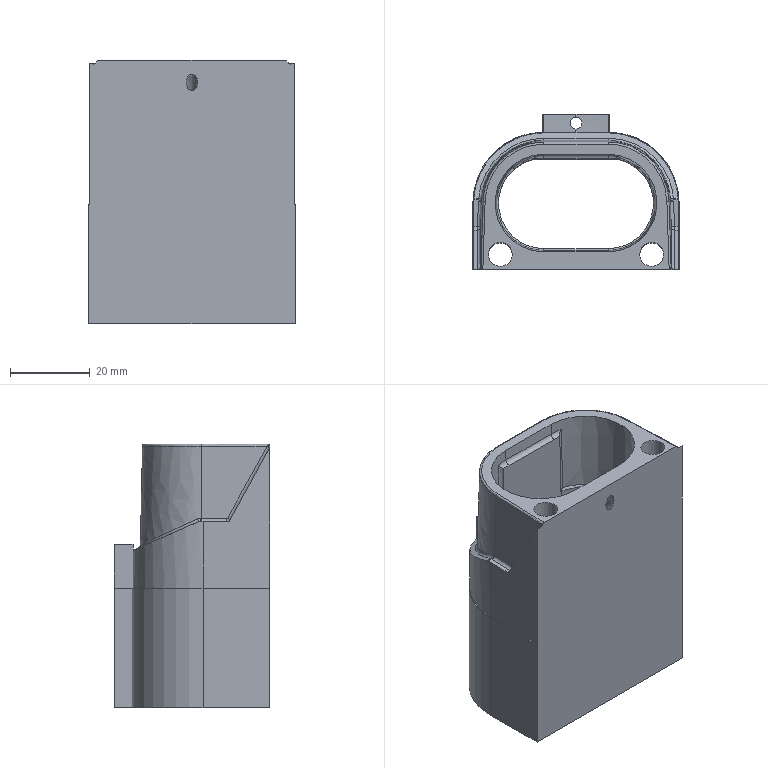Part | STEP file | lll_id62_x_t | 1 solid | 84 faces | box 51.763 x 39.033 x 66.18 mm | volume 50853 mm3 | plane 28 | spline 28 | cylinder 21 | torus 4 | cone 3 | commonest cylinder face diameters 2.008 x4 35.14 x4 0.602 x2 1.004 x2 6 x2 22.83 x2